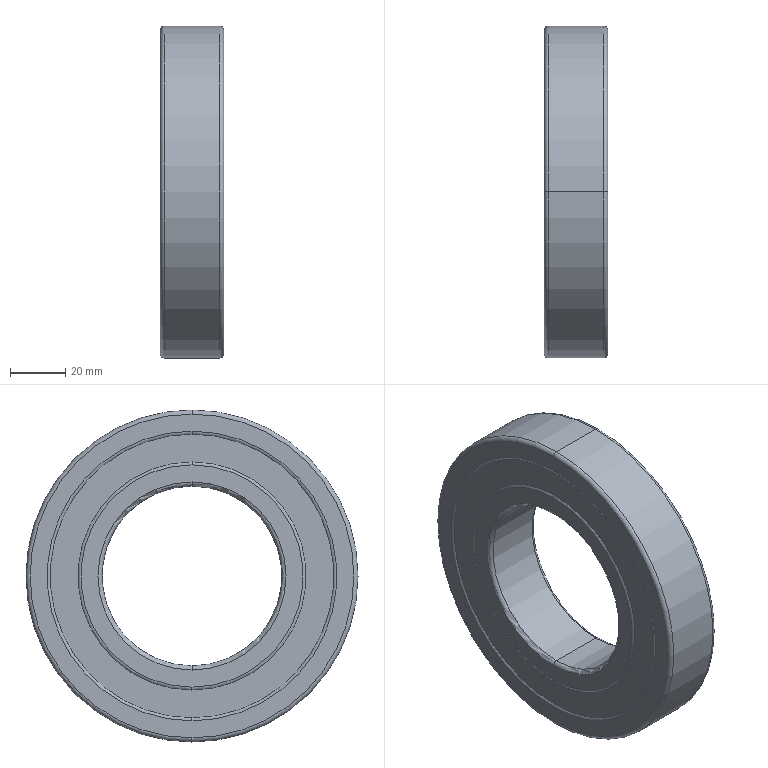Part | SolidWorks | features BaseBody 19 | 19 solids | 218 faces | box 23 x 120 x 120 mm | volume 144421 mm3 | cylinder 78 | sphere 72 | plane 42 | torus 26 | commonest cylinder face diameters 89.75 x33 95.25 x33 83.333 x4 101.667 x4 65 x2 120 x2